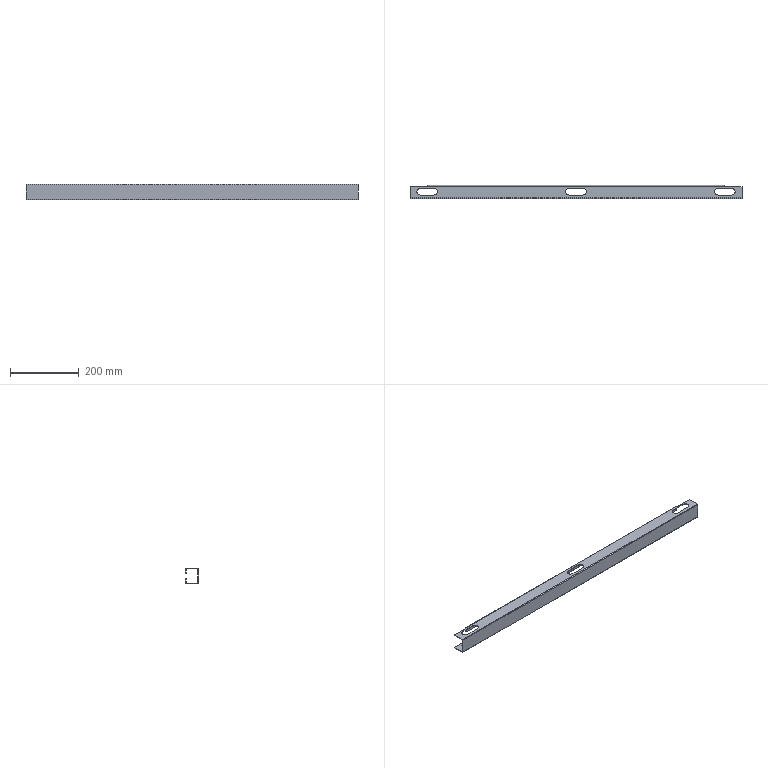Part | SolidWorks | features Cut 1, FlatPattern 1, ICE 1, SMBaseFlange 1, SheetMetal 1 | 1 solid | 70 faces | box 969 x 38 x 46 mm | volume 194985 mm3 | plane 50 | cylinder 20 | commonest cylinder face diameters 20 x12 0.4 x4 3.4 x4